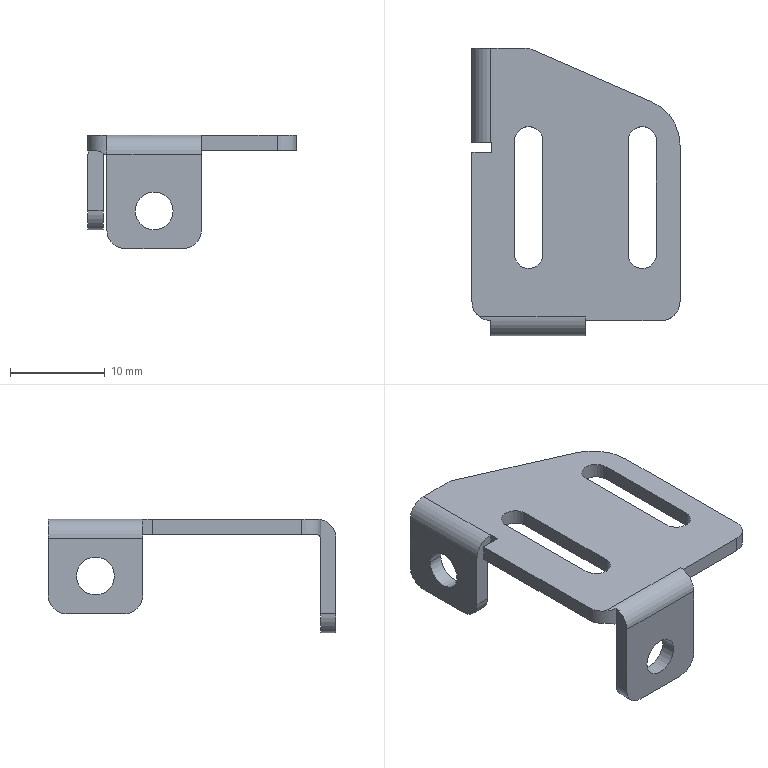Part | STEP file | ASND-0110-SDS_8 | 1 solid | 43 faces | box 22 x 30.4 x 12 mm | volume 1042 mm3 | plane 23 | cylinder 20 | commonest cylinder face diameters 4 x13 3 x4 1 x2 10 x1